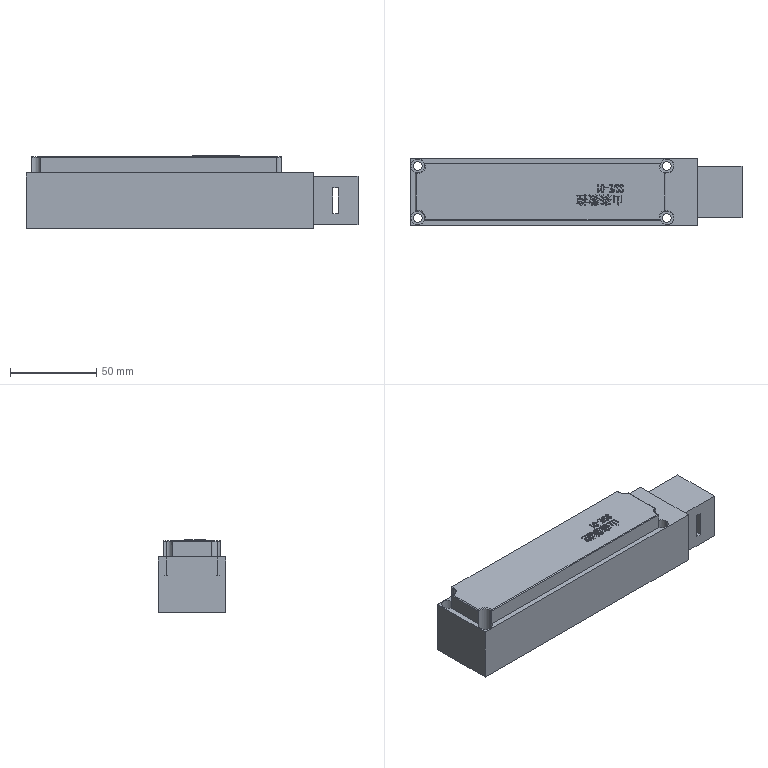Part | NX | features solid 2 | 1 solid | 336 faces | box 192 x 39 x 42 mm | volume 267690 mm3 | plane 231 | spline 81 | cylinder 19 | torus 5 | commonest cylinder face diameters 5 x8 8 x8 1 x3